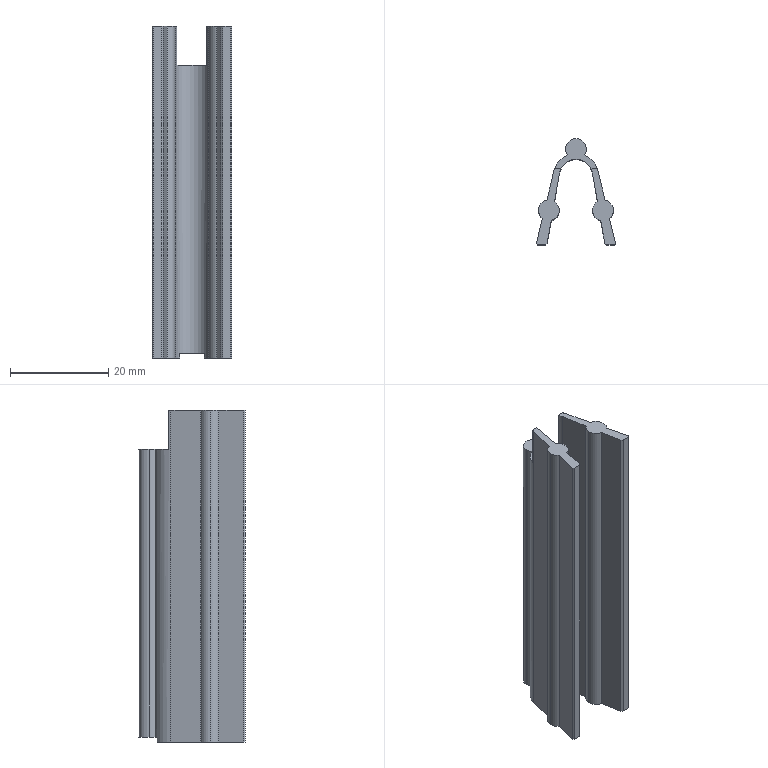Part | STEP file | slingshot push rod | 1 solid | 36 faces | box 16.072 x 21.6 x 67.5 mm | volume 5779 mm3 | plane 24 | cylinder 12 | commonest cylinder face diameters 4.2 x9 9.2 x2 6.8 x1